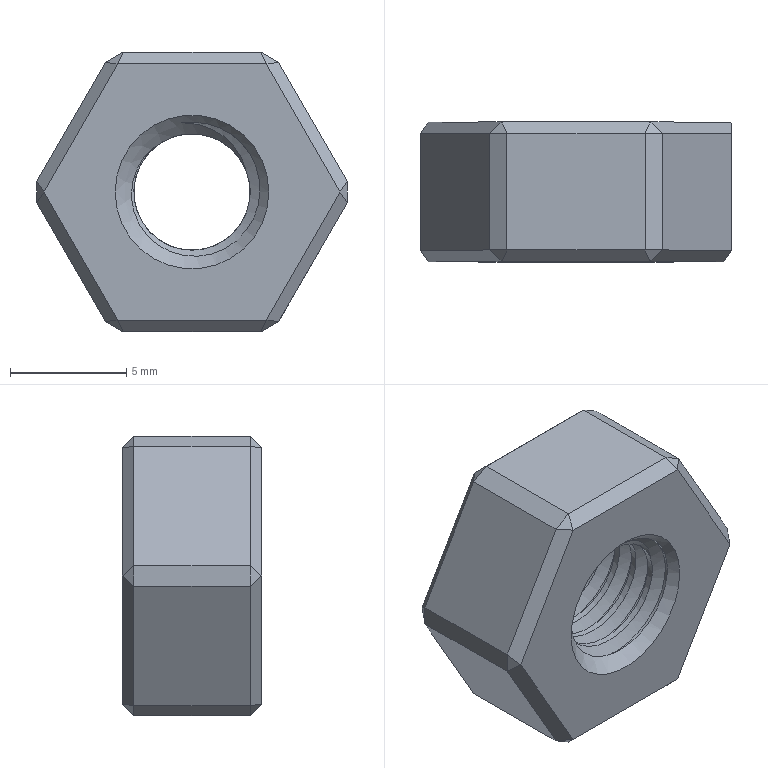Part | STEP file | Tube feed_id1826_x_t | 1 solid | 41 faces | box 13.356 x 6 x 12 mm | volume 588.844 mm3 | plane 35 | cylinder 2 | cone 2 | spline 2 | commonest cylinder face diameters 5 x1 6 x1